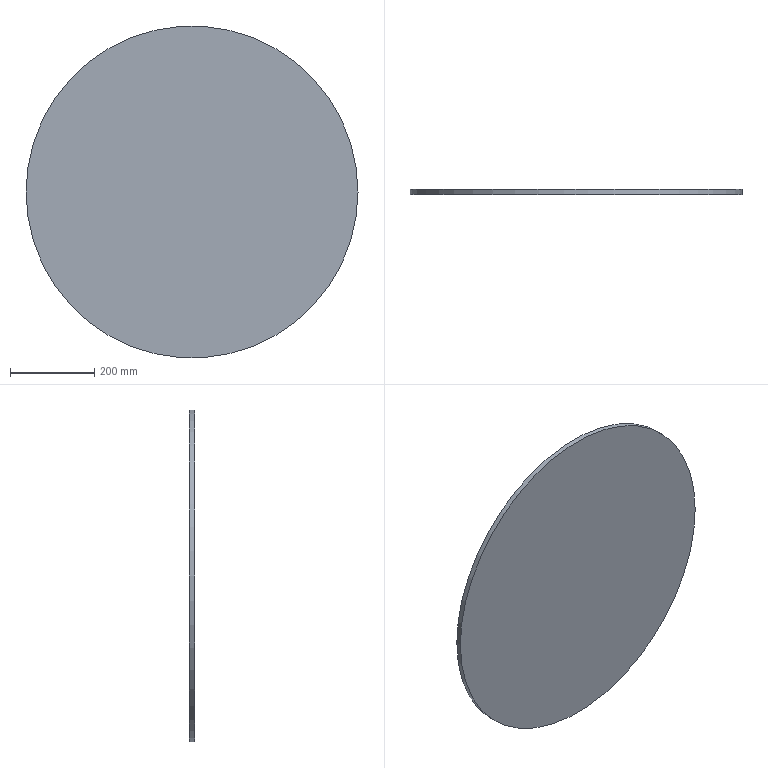Part | NX | features DATUM_CSYS 2, EXTRUDE 1, SKETCH 1 | 1 solid | 3 faces | box 790 x 12 x 790 mm | volume 5882004 mm3 | plane 2 | cylinder 1 | commonest cylinder face diameters 790 x1
STEP:
#1=CARTESIAN_POINT('',(395.,-6.,0.));
#2=VERTEX_POINT('',#1);
#3=CARTESIAN_POINT('',(0.,-6.,0.));
#4=DIRECTION('',(0.,-1.,0.));
#5=DIRECTION('',(1.,0.,0.));
#6=AXIS2_PLACEMENT_3D('',#3,#4,#5);
#7=CIRCLE('',#6,395.);
#8=EDGE_CURVE('',#2,#2,#7,.T.);
#9=ORIENTED_EDGE('',*,*,#8,.F.);
#10=EDGE_LOOP('',(#9));
#11=FACE_BOUND('',#10,.T.);
#12=CARTESIAN_POINT('',(395.,6.,0.));
#13=VERTEX_POINT('',#12);
#14=CARTESIAN_POINT('',(0.,6.,0.));
#15=DIRECTION('',(0.,-1.,0.));
#16=DIRECTION('',(1.,0.,0.));
#17=AXIS2_PLACEMENT_3D('',#14,#15,#16);
#18=CIRCLE('',#17,395.);
#19=EDGE_CURVE('',#13,#13,#18,.T.);
#20=ORIENTED_EDGE('',*,*,#19,.T.);
#21=EDGE_LOOP('',(#20));
#22=FACE_BOUND('',#21,.T.);
#23=CARTESIAN_POINT('',(0.,-6.,0.));
#24=DIRECTION('',(0.,1.,0.));
#25=DIRECTION('',(0.,0.,1.));
#26=AXIS2_PLACEMENT_3D('',#23,#24,#25);
#27=CYLINDRICAL_SURFACE('',#26,395.);
#28=ADVANCED_FACE('',(#11,#22),#27,.T.);
#29=ORIENTED_EDGE('',*,*,#8,.T.);
#30=EDGE_LOOP('',(#29));
#31=FACE_BOUND('',#30,.T.);
#32=CARTESIAN_POINT('',(0.,-6.,0.));
#33=DIRECTION('',(0.,-1.,0.));
#34=DIRECTION('',(0.,0.,-1.));
#35=AXIS2_PLACEMENT_3D('',#32,#33,#34);
#36=PLANE('',#35);
#37=ADVANCED_FACE('',(#31),#36,.T.);
#38=ORIENTED_EDGE('',*,*,#19,.F.);
#39=EDGE_LOOP('',(#38));
#40=FACE_BOUND('',#39,.T.);
#41=CARTESIAN_POINT('',(0.,6.,0.));
#42=DIRECTION('',(0.,-1.,0.));
#43=DIRECTION('',(0.,0.,-1.));
#44=AXIS2_PLACEMENT_3D('',#41,#42,#43);
#45=PLANE('',#44);
#46=ADVANCED_FACE('',(#40),#45,.F.);
#47=CLOSED_SHELL('',(#28,#37,#46));
#48=MANIFOLD_SOLID_BREP('',#47);
#49=(LENGTH_UNIT()NAMED_UNIT(*)SI_UNIT(.MILLI.,.METRE.));
#50=UNCERTAINTY_MEASURE_WITH_UNIT(LENGTH_MEASURE(0.00001),#49,'','');
#51=(NAMED_UNIT(*)PLANE_ANGLE_UNIT()SI_UNIT($,.RADIAN.));
#52=(NAMED_UNIT(*)SI_UNIT($,.STERADIAN.)SOLID_ANGLE_UNIT());
#53=(GEOMETRIC_REPRESENTATION_CONTEXT(3)GLOBAL_UNCERTAINTY_ASSIGNED_CONTEXT((#50))GLOBAL_UNIT_ASSIGNED_CONTEXT((#49,#51,#52))REPRESENTATION_CONTEXT('',''));
#54=ADVANCED_BREP_SHAPE_REPRESENTATION('',(#48),#53);